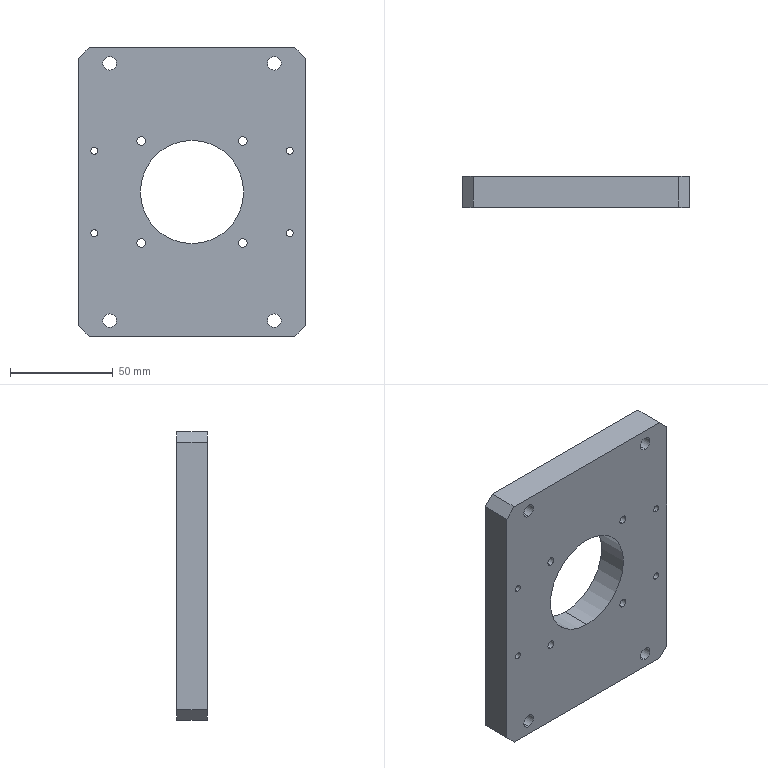Part | SolidWorks | features BaseBody 1 | 1 solid | 48 faces | box 110 x 15 x 140 mm | volume 195510 mm3 | cylinder 34 | plane 14 | commonest cylinder face diameters 3.3 x8 4.2 x8 6.6 x8 11 x8 50.2 x2
STEP:
#1=CARTESIAN_POINT('',(-47.5,0.,-21.65));
#2=VERTEX_POINT('',#1);
#3=CARTESIAN_POINT('',(-47.5,0.,-18.35));
#4=VERTEX_POINT('',#3);
#5=CARTESIAN_POINT('',(-47.5,0.,-20.));
#6=DIRECTION('',(0.,1.,0.));
#7=DIRECTION('',(0.,0.,1.));
#8=AXIS2_PLACEMENT_3D('',#5,#6,#7);
#9=CIRCLE('',#8,1.65);
#10=EDGE_CURVE('',#2,#4,#9,.T.);
#11=ORIENTED_EDGE('',*,*,#10,.F.);
#12=CARTESIAN_POINT('',(-47.5,15.,-21.65));
#13=VERTEX_POINT('',#12);
#14=CARTESIAN_POINT('',(-47.5,15.,-21.65));
#15=DIRECTION('',(0.,1.,0.));
#16=VECTOR('',#15,1000.);
#17=LINE('',#14,#16);
#18=EDGE_CURVE('',#2,#13,#17,.T.);
#19=ORIENTED_EDGE('',*,*,#18,.T.);
#20=CARTESIAN_POINT('',(-47.5,15.,-18.35));
#21=VERTEX_POINT('',#20);
#22=CARTESIAN_POINT('',(-47.5,15.,-20.));
#23=DIRECTION('',(0.,1.,0.));
#24=DIRECTION('',(0.,0.,1.));
#25=AXIS2_PLACEMENT_3D('',#22,#23,#24);
#26=CIRCLE('',#25,1.65);
#27=EDGE_CURVE('',#13,#21,#26,.T.);
#28=ORIENTED_EDGE('',*,*,#27,.T.);
#29=CARTESIAN_POINT('',(-47.5,15.,-18.35));
#30=DIRECTION('',(0.,1.,0.));
#31=VECTOR('',#30,1000.);
#32=LINE('',#29,#31);
#33=EDGE_CURVE('',#4,#21,#32,.T.);
#34=ORIENTED_EDGE('',*,*,#33,.F.);
#35=EDGE_LOOP('',(#11,#19,#28,#34));
#36=FACE_OUTER_BOUND('',#35,.T.);
#37=CARTESIAN_POINT('',(-47.5,15.,-20.));
#38=DIRECTION('',(0.,1.,0.));
#39=DIRECTION('',(0.,0.,1.));
#40=AXIS2_PLACEMENT_3D('',#37,#38,#39);
#41=CYLINDRICAL_SURFACE('',#40,1.65);
#42=ADVANCED_FACE('',(#36),#41,.F.);
#43=CARTESIAN_POINT('',(47.5,0.,-21.65));
#44=VERTEX_POINT('',#43);
#45=CARTESIAN_POINT('',(47.5,0.,-18.35));
#46=VERTEX_POINT('',#45);
#47=CARTESIAN_POINT('',(47.5,0.,-20.));
#48=DIRECTION('',(0.,1.,0.));
#49=DIRECTION('',(0.,0.,1.));
#50=AXIS2_PLACEMENT_3D('',#47,#48,#49);
#51=CIRCLE('',#50,1.65);
#52=EDGE_CURVE('',#44,#46,#51,.T.);
#53=ORIENTED_EDGE('',*,*,#52,.F.);
#54=CARTESIAN_POINT('',(47.5,15.,-21.65));
#55=VERTEX_POINT('',#54);
#56=CARTESIAN_POINT('',(47.5,15.,-21.65));
#57=DIRECTION('',(0.,1.,0.));
#58=VECTOR('',#57,1000.);
#59=LINE('',#56,#58);
#60=EDGE_CURVE('',#44,#55,#59,.T.);
#61=ORIENTED_EDGE('',*,*,#60,.T.);
#62=CARTESIAN_POINT('',(47.5,15.,-18.35));
#63=VERTEX_POINT('',#62);
#64=CARTESIAN_POINT('',(47.5,15.,-20.));
#65=DIRECTION('',(0.,1.,0.));
#66=DIRECTION('',(0.,0.,1.));
#67=AXIS2_PLACEMENT_3D('',#64,#65,#66);
#68=CIRCLE('',#67,1.65);
#69=EDGE_CURVE('',#55,#63,#68,.T.);
#70=ORIENTED_EDGE('',*,*,#69,.T.);
#71=CARTESIAN_POINT('',(47.5,15.,-18.35));
#72=DIRECTION('',(0.,1.,0.));
#73=VECTOR('',#72,1000.);
#74=LINE('',#71,#73);
#75=EDGE_CURVE('',#46,#63,#74,.T.);
#76=ORIENTED_EDGE('',*,*,#75,.F.);
#77=EDGE_LOOP('',(#53,#61,#70,#76));
#78=FACE_OUTER_BOUND('',#77,.T.);
#79=CARTESIAN_POINT('',(47.5,15.,-20.));
#80=DIRECTION('',(0.,1.,0.));
#81=DIRECTION('',(0.,0.,1.));
#82=AXIS2_PLACEMENT_3D('',#79,#80,#81);
#83=CYLINDRICAL_SURFACE('',#82,1.65);
#84=ADVANCED_FACE('',(#78),#83,.F.);
#85=CARTESIAN_POINT('',(-47.5,0.,18.35));
#86=VERTEX_POINT('',#85);
#87=CARTESIAN_POINT('',(-47.5,0.,21.65));
#88=VERTEX_POINT('',#87);
#89=CARTESIAN_POINT('',(-47.5,0.,20.));
#90=DIRECTION('',(0.,1.,0.));
#91=DIRECTION('',(0.,0.,1.));
#92=AXIS2_PLACEMENT_3D('',#89,#90,#91);
#93=CIRCLE('',#92,1.65);
#94=EDGE_CURVE('',#86,#88,#93,.T.);
#95=ORIENTED_EDGE('',*,*,#94,.F.);
#96=CARTESIAN_POINT('',(-47.5,15.,18.35));
#97=VERTEX_POINT('',#96);
#98=CARTESIAN_POINT('',(-47.5,15.,18.35));
#99=DIRECTION('',(0.,1.,0.));
#100=VECTOR('',#99,1000.);
#101=LINE('',#98,#100);
#102=EDGE_CURVE('',#86,#97,#101,.T.);
#103=ORIENTED_EDGE('',*,*,#102,.T.);
#104=CARTESIAN_POINT('',(-47.5,15.,21.65));
#105=VERTEX_POINT('',#104);
#106=CARTESIAN_POINT('',(-47.5,15.,20.));
#107=DIRECTION('',(0.,1.,0.));
#108=DIRECTION('',(0.,0.,1.));
#109=AXIS2_PLACEMENT_3D('',#106,#107,#108);
#110=CIRCLE('',#109,1.65);
#111=EDGE_CURVE('',#97,#105,#110,.T.);
#112=ORIENTED_EDGE('',*,*,#111,.T.);
#113=CARTESIAN_POINT('',(-47.5,15.,21.65));
#114=DIRECTION('',(0.,1.,0.));
#115=VECTOR('',#114,1000.);
#116=LINE('',#113,#115);
#117=EDGE_CURVE('',#88,#105,#116,.T.);
#118=ORIENTED_EDGE('',*,*,#117,.F.);
#119=EDGE_LOOP('',(#95,#103,#112,#118));
#120=FACE_OUTER_BOUND('',#119,.T.);
#121=CARTESIAN_POINT('',(-47.5,15.,20.));
#122=DIRECTION('',(0.,1.,0.));
#123=DIRECTION('',(0.,0.,1.));
#124=AXIS2_PLACEMENT_3D('',#121,#122,#123);
#125=CYLINDRICAL_SURFACE('',#124,1.65);
#126=ADVANCED_FACE('',(#120),#125,.F.);
#127=CARTESIAN_POINT('',(47.5,0.,18.35));
#128=VERTEX_POINT('',#127);
#129=CARTESIAN_POINT('',(47.5,0.,21.65));
#130=VERTEX_POINT('',#129);
#131=CARTESIAN_POINT('',(47.5,0.,20.));
#132=DIRECTION('',(0.,1.,0.));
#133=DIRECTION('',(0.,0.,1.));
#134=AXIS2_PLACEMENT_3D('',#131,#132,#133);
#135=CIRCLE('',#134,1.65);
#136=EDGE_CURVE('',#128,#130,#135,.T.);
#137=ORIENTED_EDGE('',*,*,#136,.F.);
#138=CARTESIAN_POINT('',(47.5,15.,18.35));
#139=VERTEX_POINT('',#138);
#140=CARTESIAN_POINT('',(47.5,15.,18.35));
#141=DIRECTION('',(0.,1.,0.));
#142=VECTOR('',#141,1000.);
#143=LINE('',#140,#142);
#144=EDGE_CURVE('',#128,#139,#143,.T.);
#145=ORIENTED_EDGE('',*,*,#144,.T.);
#146=CARTESIAN_POINT('',(47.5,15.,21.65));
#147=VERTEX_POINT('',#146);
#148=CARTESIAN_POINT('',(47.5,15.,20.));
#149=DIRECTION('',(0.,1.,0.));
#150=DIRECTION('',(0.,0.,1.));
#151=AXIS2_PLACEMENT_3D('',#148,#149,#150);
#152=CIRCLE('',#151,1.65);
#153=EDGE_CURVE('',#139,#147,#152,.T.);
#154=ORIENTED_EDGE('',*,*,#153,.T.);
#155=CARTESIAN_POINT('',(47.5,15.,21.65));
#156=DIRECTION('',(0.,1.,0.));
#157=VECTOR('',#156,1000.);
#158=LINE('',#155,#157);
#159=EDGE_CURVE('',#130,#147,#158,.T.);
#160=ORIENTED_EDGE('',*,*,#159,.F.);
#161=EDGE_LOOP('',(#137,#145,#154,#160));
#162=FACE_OUTER_BOUND('',#161,.T.);
#163=CARTESIAN_POINT('',(47.5,15.,20.));
#164=DIRECTION('',(0.,1.,0.));
#165=DIRECTION('',(0.,0.,1.));
#166=AXIS2_PLACEMENT_3D('',#163,#164,#165);
#167=CYLINDRICAL_SURFACE('',#166,1.65);
#168=ADVANCED_FACE('',(#162),#167,.F.);
#169=CARTESIAN_POINT('',(-40.,8.2,-68.));
#170=VERTEX_POINT('',#169);
#171=CARTESIAN_POINT('',(-40.,8.2,-57.));
#172=VERTEX_POINT('',#171);
#173=CARTESIAN_POINT('',(-40.,8.2,-62.5));
#174=DIRECTION('',(0.,1.,0.));
#175=DIRECTION('',(0.,0.,1.));
#176=AXIS2_PLACEMENT_3D('',#173,#174,#175);
#177=CIRCLE('',#176,5.5);
#178=EDGE_CURVE('',#170,#172,#177,.T.);
#179=ORIENTED_EDGE('',*,*,#178,.F.);
#180=CARTESIAN_POINT('',(-40.,15.,-68.));
#181=VERTEX_POINT('',#180);
#182=CARTESIAN_POINT('',(-40.,15.,-68.));
#183=DIRECTION('',(0.,1.,0.));
#184=VECTOR('',#183,1000.);
#185=LINE('',#182,#184);
#186=EDGE_CURVE('',#170,#181,#185,.T.);
#187=ORIENTED_EDGE('',*,*,#186,.T.);
#188=CARTESIAN_POINT('',(-40.,15.,-57.));
#189=VERTEX_POINT('',#188);
#190=CARTESIAN_POINT('',(-40.,15.,-62.5));
#191=DIRECTION('',(0.,1.,0.));
#192=DIRECTION('',(0.,0.,1.));
#193=AXIS2_PLACEMENT_3D('',#190,#191,#192);
#194=CIRCLE('',#193,5.5);
#195=EDGE_CURVE('',#181,#189,#194,.T.);
#196=ORIENTED_EDGE('',*,*,#195,.T.);
#197=CARTESIAN_POINT('',(-40.,15.,-57.));
#198=DIRECTION('',(0.,1.,0.));
#199=VECTOR('',#198,1000.);
#200=LINE('',#197,#199);
#201=EDGE_CURVE('',#172,#189,#200,.T.);
#202=ORIENTED_EDGE('',*,*,#201,.F.);
#203=EDGE_LOOP('',(#179,#187,#196,#202));
#204=FACE_OUTER_BOUND('',#203,.T.);
#205=CARTESIAN_POINT('',(-40.,15.,-62.5));
#206=DIRECTION('',(0.,1.,0.));
#207=DIRECTION('',(0.,0.,1.));
#208=AXIS2_PLACEMENT_3D('',#205,#206,#207);
#209=CYLINDRICAL_SURFACE('',#208,5.5);
#210=ADVANCED_FACE('',(#204),#209,.F.);
#211=CARTESIAN_POINT('',(-40.,0.,-65.8));
#212=VERTEX_POINT('',#211);
#213=CARTESIAN_POINT('',(-40.,0.,-59.2));
#214=VERTEX_POINT('',#213);
#215=CARTESIAN_POINT('',(-40.,0.,-62.5));
#216=DIRECTION('',(0.,1.,0.));
#217=DIRECTION('',(0.,0.,1.));
#218=AXIS2_PLACEMENT_3D('',#215,#216,#217);
#219=CIRCLE('',#218,3.3);
#220=EDGE_CURVE('',#212,#214,#219,.T.);
#221=ORIENTED_EDGE('',*,*,#220,.F.);
#222=CARTESIAN_POINT('',(-40.,8.2,-65.8));
#223=VERTEX_POINT('',#222);
#224=CARTESIAN_POINT('',(-40.,15.,-65.8));
#225=DIRECTION('',(0.,1.,0.));
#226=VECTOR('',#225,1000.);
#227=LINE('',#224,#226);
#228=EDGE_CURVE('',#212,#223,#227,.T.);
#229=ORIENTED_EDGE('',*,*,#228,.T.);
#230=CARTESIAN_POINT('',(-40.,8.2,-59.2));
#231=VERTEX_POINT('',#230);
#232=CARTESIAN_POINT('',(-40.,8.2,-62.5));
#233=DIRECTION('',(0.,1.,0.));
#234=DIRECTION('',(0.,0.,1.));
#235=AXIS2_PLACEMENT_3D('',#232,#233,#234);
#236=CIRCLE('',#235,3.3);
#237=EDGE_CURVE('',#223,#231,#236,.T.);
#238=ORIENTED_EDGE('',*,*,#237,.T.);
#239=CARTESIAN_POINT('',(-40.,15.,-59.2));
#240=DIRECTION('',(0.,1.,0.));
#241=VECTOR('',#240,1000.);
#242=LINE('',#239,#241);
#243=EDGE_CURVE('',#214,#231,#242,.T.);
#244=ORIENTED_EDGE('',*,*,#243,.F.);
#245=EDGE_LOOP('',(#221,#229,#238,#244));
#246=FACE_OUTER_BOUND('',#245,.T.);
#247=CARTESIAN_POINT('',(-40.,15.,-62.5));
#248=DIRECTION('',(0.,1.,0.));
#249=DIRECTION('',(0.,0.,1.));
#250=AXIS2_PLACEMENT_3D('',#247,#248,#249);
#251=CYLINDRICAL_SURFACE('',#250,3.3);
#252=ADVANCED_FACE('',(#246),#251,.F.);
#253=CARTESIAN_POINT('',(-40.,8.2,57.));
#254=VERTEX_POINT('',#253);
#255=CARTESIAN_POINT('',(-40.,8.2,68.));
#256=VERTEX_POINT('',#255);
#257=CARTESIAN_POINT('',(-40.,8.2,62.5));
#258=DIRECTION('',(0.,1.,0.));
#259=DIRECTION('',(0.,0.,1.));
#260=AXIS2_PLACEMENT_3D('',#257,#258,#259);
#261=CIRCLE('',#260,5.5);
#262=EDGE_CURVE('',#254,#256,#261,.T.);
#263=ORIENTED_EDGE('',*,*,#262,.F.);
#264=CARTESIAN_POINT('',(-40.,15.,57.));
#265=VERTEX_POINT('',#264);
#266=CARTESIAN_POINT('',(-40.,15.,57.));
#267=DIRECTION('',(0.,1.,0.));
#268=VECTOR('',#267,1000.);
#269=LINE('',#266,#268);
#270=EDGE_CURVE('',#254,#265,#269,.T.);
#271=ORIENTED_EDGE('',*,*,#270,.T.);
#272=CARTESIAN_POINT('',(-40.,15.,68.));
#273=VERTEX_POINT('',#272);
#274=CARTESIAN_POINT('',(-40.,15.,62.5));
#275=DIRECTION('',(0.,1.,0.));
#276=DIRECTION('',(0.,0.,1.));
#277=AXIS2_PLACEMENT_3D('',#274,#275,#276);
#278=CIRCLE('',#277,5.5);
#279=EDGE_CURVE('',#265,#273,#278,.T.);
#280=ORIENTED_EDGE('',*,*,#279,.T.);
#281=CARTESIAN_POINT('',(-40.,15.,68.));
#282=DIRECTION('',(0.,1.,0.));
#283=VECTOR('',#282,1000.);
#284=LINE('',#281,#283);
#285=EDGE_CURVE('',#256,#273,#284,.T.);
#286=ORIENTED_EDGE('',*,*,#285,.F.);
#287=EDGE_LOOP('',(#263,#271,#280,#286));
#288=FACE_OUTER_BOUND('',#287,.T.);
#289=CARTESIAN_POINT('',(-40.,15.,62.5));
#290=DIRECTION('',(0.,1.,0.));
#291=DIRECTION('',(0.,0.,1.));
#292=AXIS2_PLACEMENT_3D('',#289,#290,#291);
#293=CYLINDRICAL_SURFACE('',#292,5.5);
#294=ADVANCED_FACE('',(#288),#293,.F.);
#295=CARTESIAN_POINT('',(-40.,0.,59.2));
#296=VERTEX_POINT('',#295);
#297=CARTESIAN_POINT('',(-40.,0.,65.8));
#298=VERTEX_POINT('',#297);
#299=CARTESIAN_POINT('',(-40.,0.,62.5));
#300=DIRECTION('',(0.,1.,0.));
#301=DIRECTION('',(0.,0.,1.));
#302=AXIS2_PLACEMENT_3D('',#299,#300,#301);
#303=CIRCLE('',#302,3.3);
#304=EDGE_CURVE('',#296,#298,#303,.T.);
#305=ORIENTED_EDGE('',*,*,#304,.F.);
#306=CARTESIAN_POINT('',(-40.,8.2,59.2));
#307=VERTEX_POINT('',#306);
#308=CARTESIAN_POINT('',(-40.,15.,59.2));
#309=DIRECTION('',(0.,1.,0.));
#310=VECTOR('',#309,1000.);
#311=LINE('',#308,#310);
#312=EDGE_CURVE('',#296,#307,#311,.T.);
#313=ORIENTED_EDGE('',*,*,#312,.T.);
#314=CARTESIAN_POINT('',(-40.,8.2,65.8));
#315=VERTEX_POINT('',#314);
#316=CARTESIAN_POINT('',(-40.,8.2,62.5));
#317=DIRECTION('',(0.,1.,0.));
#318=DIRECTION('',(0.,0.,1.));
#319=AXIS2_PLACEMENT_3D('',#316,#317,#318);
#320=CIRCLE('',#319,3.3);
#321=EDGE_CURVE('',#307,#315,#320,.T.);
#322=ORIENTED_EDGE('',*,*,#321,.T.);
#323=CARTESIAN_POINT('',(-40.,15.,65.8));
#324=DIRECTION('',(0.,1.,0.));
#325=VECTOR('',#324,1000.);
#326=LINE('',#323,#325);
#327=EDGE_CURVE('',#298,#315,#326,.T.);
#328=ORIENTED_EDGE('',*,*,#327,.F.);
#329=EDGE_LOOP('',(#305,#313,#322,#328));
#330=FACE_OUTER_BOUND('',#329,.T.);
#331=CARTESIAN_POINT('',(-40.,15.,62.5));
#332=DIRECTION('',(0.,1.,0.));
#333=DIRECTION('',(0.,0.,1.));
#334=AXIS2_PLACEMENT_3D('',#331,#332,#333);
#335=CYLINDRICAL_SURFACE('',#334,3.3);
#336=ADVANCED_FACE('',(#330),#335,.F.);
#337=CARTESIAN_POINT('',(40.,8.2,57.));
#338=VERTEX_POINT('',#337);
#339=CARTESIAN_POINT('',(40.,8.2,68.));
#340=VERTEX_POINT('',#339);
#341=CARTESIAN_POINT('',(40.,8.2,62.5));
#342=DIRECTION('',(0.,1.,0.));
#343=DIRECTION('',(0.,0.,1.));
#344=AXIS2_PLACEMENT_3D('',#341,#342,#343);
#345=CIRCLE('',#344,5.5);
#346=EDGE_CURVE('',#338,#340,#345,.T.);
#347=ORIENTED_EDGE('',*,*,#346,.F.);
#348=CARTESIAN_POINT('',(40.,15.,57.));
#349=VERTEX_POINT('',#348);
#350=CARTESIAN_POINT('',(40.,15.,57.));
#351=DIRECTION('',(0.,1.,0.));
#352=VECTOR('',#351,1000.);
#353=LINE('',#350,#352);
#354=EDGE_CURVE('',#338,#349,#353,.T.);
#355=ORIENTED_EDGE('',*,*,#354,.T.);
#356=CARTESIAN_POINT('',(40.,15.,68.));
#357=VERTEX_POINT('',#356);
#358=CARTESIAN_POINT('',(40.,15.,62.5));
#359=DIRECTION('',(0.,1.,0.));
#360=DIRECTION('',(0.,0.,1.));
#361=AXIS2_PLACEMENT_3D('',#358,#359,#360);
#362=CIRCLE('',#361,5.5);
#363=EDGE_CURVE('',#349,#357,#362,.T.);
#364=ORIENTED_EDGE('',*,*,#363,.T.);
#365=CARTESIAN_POINT('',(40.,15.,68.));
#366=DIRECTION('',(0.,1.,0.));
#367=VECTOR('',#366,1000.);
#368=LINE('',#365,#367);
#369=EDGE_CURVE('',#340,#357,#368,.T.);
#370=ORIENTED_EDGE('',*,*,#369,.F.);
#371=EDGE_LOOP('',(#347,#355,#364,#370));
#372=FACE_OUTER_BOUND('',#371,.T.);
#373=CARTESIAN_POINT('',(40.,15.,62.5));
#374=DIRECTION('',(0.,1.,0.));
#375=DIRECTION('',(0.,0.,1.));
#376=AXIS2_PLACEMENT_3D('',#373,#374,#375);
#377=CYLINDRICAL_SURFACE('',#376,5.5);
#378=ADVANCED_FACE('',(#372),#377,.F.);
#379=CARTESIAN_POINT('',(40.,0.,59.2));
#380=VERTEX_POINT('',#379);
#381=CARTESIAN_POINT('',(40.,0.,65.8));
#382=VERTEX_POINT('',#381);
#383=CARTESIAN_POINT('',(40.,0.,62.5));
#384=DIRECTION('',(0.,1.,0.));
#385=DIRECTION('',(0.,0.,1.));
#386=AXIS2_PLACEMENT_3D('',#383,#384,#385);
#387=CIRCLE('',#386,3.3);
#388=EDGE_CURVE('',#380,#382,#387,.T.);
#389=ORIENTED_EDGE('',*,*,#388,.F.);
#390=CARTESIAN_POINT('',(40.,8.2,59.2));
#391=VERTEX_POINT('',#390);
#392=CARTESIAN_POINT('',(40.,15.,59.2));
#393=DIRECTION('',(0.,1.,0.));
#394=VECTOR('',#393,1000.);
#395=LINE('',#392,#394);
#396=EDGE_CURVE('',#380,#391,#395,.T.);
#397=ORIENTED_EDGE('',*,*,#396,.T.);
#398=CARTESIAN_POINT('',(40.,8.2,65.8));
#399=VERTEX_POINT('',#398);
#400=CARTESIAN_POINT('',(40.,8.2,62.5));
#401=DIRECTION('',(0.,1.,0.));
#402=DIRECTION('',(0.,0.,1.));
#403=AXIS2_PLACEMENT_3D('',#400,#401,#402);
#404=CIRCLE('',#403,3.3);
#405=EDGE_CURVE('',#391,#399,#404,.T.);
#406=ORIENTED_EDGE('',*,*,#405,.T.);
#407=CARTESIAN_POINT('',(40.,15.,65.8));
#408=DIRECTION('',(0.,1.,0.));
#409=VECTOR('',#408,1000.);
#410=LINE('',#407,#409);
#411=EDGE_CURVE('',#382,#399,#410,.T.);
#412=ORIENTED_EDGE('',*,*,#411,.F.);
#413=EDGE_LOOP('',(#389,#397,#406,#412));
#414=FACE_OUTER_BOUND('',#413,.T.);
#415=CARTESIAN_POINT('',(40.,15.,62.5));
#416=DIRECTION('',(0.,1.,0.));
#417=DIRECTION('',(0.,0.,1.));
#418=AXIS2_PLACEMENT_3D('',#415,#416,#417);
#419=CYLINDRICAL_SURFACE('',#418,3.3);
#420=ADVANCED_FACE('',(#414),#419,.F.);
#421=CARTESIAN_POINT('',(40.,8.2,-68.));
#422=VERTEX_POINT('',#421);
#423=CARTESIAN_POINT('',(40.,8.2,-57.));
#424=VERTEX_POINT('',#423);
#425=CARTESIAN_POINT('',(40.,8.2,-62.5));
#426=DIRECTION('',(0.,1.,0.));
#427=DIRECTION('',(0.,0.,1.));
#428=AXIS2_PLACEMENT_3D('',#425,#426,#427);
#429=CIRCLE('',#428,5.5);
#430=EDGE_CURVE('',#422,#424,#429,.T.);
#431=ORIENTED_EDGE('',*,*,#430,.F.);
#432=CARTESIAN_POINT('',(40.,15.,-68.));
#433=VERTEX_POINT('',#432);
#434=CARTESIAN_POINT('',(40.,15.,-68.));
#435=DIRECTION('',(0.,1.,0.));
#436=VECTOR('',#435,1000.);
#437=LINE('',#434,#436);
#438=EDGE_CURVE('',#422,#433,#437,.T.);
#439=ORIENTED_EDGE('',*,*,#438,.T.);
#440=CARTESIAN_POINT('',(40.,15.,-57.));
#441=VERTEX_POINT('',#440);
#442=CARTESIAN_POINT('',(40.,15.,-62.5));
#443=DIRECTION('',(0.,1.,0.));
#444=DIRECTION('',(0.,0.,1.));
#445=AXIS2_PLACEMENT_3D('',#442,#443,#444);
#446=CIRCLE('',#445,5.5);
#447=EDGE_CURVE('',#433,#441,#446,.T.);
#448=ORIENTED_EDGE('',*,*,#447,.T.);
#449=CARTESIAN_POINT('',(40.,15.,-57.));
#450=DIRECTION('',(0.,1.,0.));
#451=VECTOR('',#450,1000.);
#452=LINE('',#449,#451);
#453=EDGE_CURVE('',#424,#441,#452,.T.);
#454=ORIENTED_EDGE('',*,*,#453,.F.);
#455=EDGE_LOOP('',(#431,#439,#448,#454));
#456=FACE_OUTER_BOUND('',#455,.T.);
#457=CARTESIAN_POINT('',(40.,15.,-62.5));
#458=DIRECTION('',(0.,1.,0.));
#459=DIRECTION('',(0.,0.,1.));
#460=AXIS2_PLACEMENT_3D('',#457,#458,#459);
#461=CYLINDRICAL_SURFACE('',#460,5.5);
#462=ADVANCED_FACE('',(#456),#461,.F.);
#463=CARTESIAN_POINT('',(40.,0.,-65.8));
#464=VERTEX_POINT('',#463);
#465=CARTESIAN_POINT('',(40.,0.,-59.2));
#466=VERTEX_POINT('',#465);
#467=CARTESIAN_POINT('',(40.,0.,-62.5));
#468=DIRECTION('',(0.,1.,0.));
#469=DIRECTION('',(0.,0.,1.));
#470=AXIS2_PLACEMENT_3D('',#467,#468,#469);
#471=CIRCLE('',#470,3.3);
#472=EDGE_CURVE('',#464,#466,#471,.T.);
#473=ORIENTED_EDGE('',*,*,#472,.F.);
#474=CARTESIAN_POINT('',(40.,8.2,-65.8));
#475=VERTEX_POINT('',#474);
#476=CARTESIAN_POINT('',(40.,15.,-65.8));
#477=DIRECTION('',(0.,1.,0.));
#478=VECTOR('',#477,1000.);
#479=LINE('',#476,#478);
#480=EDGE_CURVE('',#464,#475,#479,.T.);
#481=ORIENTED_EDGE('',*,*,#480,.T.);
#482=CARTESIAN_POINT('',(40.,8.2,-59.2));
#483=VERTEX_POINT('',#482);
#484=CARTESIAN_POINT('',(40.,8.2,-62.5));
#485=DIRECTION('',(0.,1.,0.));
#486=DIRECTION('',(0.,0.,1.));
#487=AXIS2_PLACEMENT_3D('',#484,#485,#486);
#488=CIRCLE('',#487,3.3);
#489=EDGE_CURVE('',#475,#483,#488,.T.);
#490=ORIENTED_EDGE('',*,*,#489,.T.);
#491=CARTESIAN_POINT('',(40.,15.,-59.2));
#492=DIRECTION('',(0.,1.,0.));
#493=VECTOR('',#492,1000.);
#494=LINE('',#491,#493);
#495=EDGE_CURVE('',#466,#483,#494,.T.);
#496=ORIENTED_EDGE('',*,*,#495,.F.);
#497=EDGE_LOOP('',(#473,#481,#490,#496));
#498=FACE_OUTER_BOUND('',#497,.T.);
#499=CARTESIAN_POINT('',(40.,15.,-62.5));
#500=DIRECTION('',(0.,1.,0.));
#501=DIRECTION('',(0.,0.,1.));
#502=AXIS2_PLACEMENT_3D('',#499,#500,#501);
#503=CYLINDRICAL_SURFACE('',#502,3.3);
#504=ADVANCED_FACE('',(#498),#503,.F.);
#505=CARTESIAN_POINT('',(-24.749,0.,-26.849));
#506=VERTEX_POINT('',#505);
#507=CARTESIAN_POINT('',(-24.749,0.,-22.649));
#508=VERTEX_POINT('',#507);
#509=CARTESIAN_POINT('',(-24.749,0.,-24.749));
#510=DIRECTION('',(0.,1.,0.));
#511=DIRECTION('',(0.,0.,1.));
#512=AXIS2_PLACEMENT_3D('',#509,#510,#511);
#513=CIRCLE('',#512,2.1);
#514=EDGE_CURVE('',#506,#508,#513,.T.);
#515=ORIENTED_EDGE('',*,*,#514,.F.);
#516=CARTESIAN_POINT('',(-24.749,15.,-26.849));
#517=VERTEX_POINT('',#516);
#518=CARTESIAN_POINT('',(-24.749,15.,-26.849));
#519=DIRECTION('',(0.,1.,0.));
#520=VECTOR('',#519,1000.);
#521=LINE('',#518,#520);
#522=EDGE_CURVE('',#506,#517,#521,.T.);
#523=ORIENTED_EDGE('',*,*,#522,.T.);
#524=CARTESIAN_POINT('',(-24.749,15.,-22.649));
#525=VERTEX_POINT('',#524);
#526=CARTESIAN_POINT('',(-24.749,15.,-24.749));
#527=DIRECTION('',(0.,1.,0.));
#528=DIRECTION('',(0.,0.,1.));
#529=AXIS2_PLACEMENT_3D('',#526,#527,#528);
#530=CIRCLE('',#529,2.1);
#531=EDGE_CURVE('',#517,#525,#530,.T.);
#532=ORIENTED_EDGE('',*,*,#531,.T.);
#533=CARTESIAN_POINT('',(-24.749,15.,-22.649));
#534=DIRECTION('',(0.,1.,0.));
#535=VECTOR('',#534,1000.);
#536=LINE('',#533,#535);
#537=EDGE_CURVE('',#508,#525,#536,.T.);
#538=ORIENTED_EDGE('',*,*,#537,.F.);
#539=EDGE_LOOP('',(#515,#523,#532,#538));
#540=FACE_OUTER_BOUND('',#539,.T.);
#541=CARTESIAN_POINT('',(-24.749,15.,-24.749));
#542=DIRECTION('',(0.,1.,0.));
#543=DIRECTION('',(0.,0.,1.));
#544=AXIS2_PLACEMENT_3D('',#541,#542,#543);
#545=CYLINDRICAL_SURFACE('',#544,2.1);
#546=ADVANCED_FACE('',(#540),#545,.F.);
#547=CARTESIAN_POINT('',(24.749,0.,22.649));
#548=VERTEX_POINT('',#547);
#549=CARTESIAN_POINT('',(24.749,0.,26.849));
#550=VERTEX_POINT('',#549);
#551=CARTESIAN_POINT('',(24.749,0.,24.749));
#552=DIRECTION('',(0.,1.,0.));
#553=DIRECTION('',(0.,0.,1.));
#554=AXIS2_PLACEMENT_3D('',#551,#552,#553);
#555=CIRCLE('',#554,2.1);
#556=EDGE_CURVE('',#548,#550,#555,.T.);
#557=ORIENTED_EDGE('',*,*,#556,.F.);
#558=CARTESIAN_POINT('',(24.749,15.,22.649));
#559=VERTEX_POINT('',#558);
#560=CARTESIAN_POINT('',(24.749,15.,22.649));
#561=DIRECTION('',(0.,1.,0.));
#562=VECTOR('',#561,1000.);
#563=LINE('',#560,#562);
#564=EDGE_CURVE('',#548,#559,#563,.T.);
#565=ORIENTED_EDGE('',*,*,#564,.T.);
#566=CARTESIAN_POINT('',(24.749,15.,26.849));
#567=VERTEX_POINT('',#566);
#568=CARTESIAN_POINT('',(24.749,15.,24.749));
#569=DIRECTION('',(0.,1.,0.));
#570=DIRECTION('',(0.,0.,1.));
#571=AXIS2_PLACEMENT_3D('',#568,#569,#570);
#572=CIRCLE('',#571,2.1);
#573=EDGE_CURVE('',#559,#567,#572,.T.);
#574=ORIENTED_EDGE('',*,*,#573,.T.);
#575=CARTESIAN_POINT('',(24.749,15.,26.849));
#576=DIRECTION('',(0.,1.,0.));
#577=VECTOR('',#576,1000.);
#578=LINE('',#575,#577);
#579=EDGE_CURVE('',#550,#567,#578,.T.);
#580=ORIENTED_EDGE('',*,*,#579,.F.);
#581=EDGE_LOOP('',(#557,#565,#574,#580));
#582=FACE_OUTER_BOUND('',#581,.T.);
#583=CARTESIAN_POINT('',(24.749,15.,24.749));
#584=DIRECTION('',(0.,1.,0.));
#585=DIRECTION('',(0.,0.,1.));
#586=AXIS2_PLACEMENT_3D('',#583,#584,#585);
#587=CYLINDRICAL_SURFACE('',#586,2.1);
#588=ADVANCED_FACE('',(#582),#587,.F.);
#589=CARTESIAN_POINT('',(24.749,0.,-26.849));
#590=VERTEX_POINT('',#589);
#591=CARTESIAN_POINT('',(24.749,0.,-22.649));
#592=VERTEX_POINT('',#591);
#593=CARTESIAN_POINT('',(24.749,0.,-24.749));
#594=DIRECTION('',(0.,1.,0.));
#595=DIRECTION('',(0.,0.,1.));
#596=AXIS2_PLACEMENT_3D('',#593,#594,#595);
#597=CIRCLE('',#596,2.1);
#598=EDGE_CURVE('',#590,#592,#597,.T.);
#599=ORIENTED_EDGE('',*,*,#598,.F.);
#600=CARTESIAN_POINT('',(24.749,15.,-26.849));
#601=VERTEX_POINT('',#600);
#602=CARTESIAN_POINT('',(24.749,15.,-26.849));
#603=DIRECTION('',(0.,1.,0.));
#604=VECTOR('',#603,1000.);
#605=LINE('',#602,#604);
#606=EDGE_CURVE('',#590,#601,#605,.T.);
#607=ORIENTED_EDGE('',*,*,#606,.T.);
#608=CARTESIAN_POINT('',(24.749,15.,-22.649));
#609=VERTEX_POINT('',#608);
#610=CARTESIAN_POINT('',(24.749,15.,-24.749));
#611=DIRECTION('',(0.,1.,0.));
#612=DIRECTION('',(0.,0.,1.));
#613=AXIS2_PLACEMENT_3D('',#610,#611,#612);
#614=CIRCLE('',#613,2.1);
#615=EDGE_CURVE('',#601,#609,#614,.T.);
#616=ORIENTED_EDGE('',*,*,#615,.T.);
#617=CARTESIAN_POINT('',(24.749,15.,-22.649));
#618=DIRECTION('',(0.,1.,0.));
#619=VECTOR('',#618,1000.);
#620=LINE('',#617,#619);
#621=EDGE_CURVE('',#592,#609,#620,.T.);
#622=ORIENTED_EDGE('',*,*,#621,.F.);
#623=EDGE_LOOP('',(#599,#607,#616,#622));
#624=FACE_OUTER_BOUND('',#623,.T.);
#625=CARTESIAN_POINT('',(24.749,15.,-24.749));
#626=DIRECTION('',(0.,1.,0.));
#627=DIRECTION('',(0.,0.,1.));
#628=AXIS2_PLACEMENT_3D('',#625,#626,#627);
#629=CYLINDRICAL_SURFACE('',#628,2.1);
#630=ADVANCED_FACE('',(#624),#629,.F.);
#631=CARTESIAN_POINT('',(-24.749,0.,22.649));
#632=VERTEX_POINT('',#631);
#633=CARTESIAN_POINT('',(-24.749,0.,26.849));
#634=VERTEX_POINT('',#633);
#635=CARTESIAN_POINT('',(-24.749,0.,24.749));
#636=DIRECTION('',(0.,1.,0.));
#637=DIRECTION('',(0.,0.,1.));
#638=AXIS2_PLACEMENT_3D('',#635,#636,#637);
#639=CIRCLE('',#638,2.1);
#640=EDGE_CURVE('',#632,#634,#639,.T.);
#641=ORIENTED_EDGE('',*,*,#640,.F.);
#642=CARTESIAN_POINT('',(-24.749,15.,22.649));
#643=VERTEX_POINT('',#642);
#644=CARTESIAN_POINT('',(-24.749,15.,22.649));
#645=DIRECTION('',(0.,1.,0.));
#646=VECTOR('',#645,1000.);
#647=LINE('',#644,#646);
#648=EDGE_CURVE('',#632,#643,#647,.T.);
#649=ORIENTED_EDGE('',*,*,#648,.T.);
#650=CARTESIAN_POINT('',(-24.749,15.,26.849));
#651=VERTEX_POINT('',#650);
#652=CARTESIAN_POINT('',(-24.749,15.,24.749));
#653=DIRECTION('',(0.,1.,0.));
#654=DIRECTION('',(0.,0.,1.));
#655=AXIS2_PLACEMENT_3D('',#652,#653,#654);
#656=CIRCLE('',#655,2.1);
#657=EDGE_CURVE('',#643,#651,#656,.T.);
#658=ORIENTED_EDGE('',*,*,#657,.T.);
#659=CARTESIAN_POINT('',(-24.749,15.,26.849));
#660=DIRECTION('',(0.,1.,0.));
#661=VECTOR('',#660,1000.);
#662=LINE('',#659,#661);
#663=EDGE_CURVE('',#634,#651,#662,.T.);
#664=ORIENTED_EDGE('',*,*,#663,.F.);
#665=EDGE_LOOP('',(#641,#649,#658,#664));
#666=FACE_OUTER_BOUND('',#665,.T.);
#667=CARTESIAN_POINT('',(-24.749,15.,24.749));
#668=DIRECTION('',(0.,1.,0.));
#669=DIRECTION('',(0.,0.,1.));
#670=AXIS2_PLACEMENT_3D('',#667,#668,#669);
#671=CYLINDRICAL_SURFACE('',#670,2.1);
#672=ADVANCED_FACE('',(#666),#671,.F.);
#673=CARTESIAN_POINT('',(0.,0.,-25.1));
#674=VERTEX_POINT('',#673);
#675=CARTESIAN_POINT('',(0.,0.,25.1));
#676=VERTEX_POINT('',#675);
#677=CARTESIAN_POINT('',(0.,0.,0.));
#678=DIRECTION('',(0.,1.,0.));
#679=DIRECTION('',(0.,0.,1.));
#680=AXIS2_PLACEMENT_3D('',#677,#678,#679);
#681=CIRCLE('',#680,25.1);
#682=EDGE_CURVE('',#674,#676,#681,.T.);
#683=ORIENTED_EDGE('',*,*,#682,.F.);
#684=CARTESIAN_POINT('',(0.,15.,-25.1));
#685=VERTEX_POINT('',#684);
#686=CARTESIAN_POINT('',(0.,0.,-25.1));
#687=DIRECTION('',(0.,1.,0.));
#688=VECTOR('',#687,1000.);
#689=LINE('',#686,#688);
#690=EDGE_CURVE('',#674,#685,#689,.T.);
#691=ORIENTED_EDGE('',*,*,#690,.T.);
#692=CARTESIAN_POINT('',(0.,15.,25.1));
#693=VERTEX_POINT('',#692);
#694=CARTESIAN_POINT('',(0.,15.,0.));
#695=DIRECTION('',(0.,1.,0.));
#696=DIRECTION('',(0.,0.,1.));
#697=AXIS2_PLACEMENT_3D('',#694,#695,#696);
#698=CIRCLE('',#697,25.1);
#699=EDGE_CURVE('',#685,#693,#698,.T.);
#700=ORIENTED_EDGE('',*,*,#699,.T.);
#701=CARTESIAN_POINT('',(0.,0.,25.1));
#702=DIRECTION('',(0.,1.,0.));
#703=VECTOR('',#702,1000.);
#704=LINE('',#701,#703);
#705=EDGE_CURVE('',#676,#693,#704,.T.);
#706=ORIENTED_EDGE('',*,*,#705,.F.);
#707=EDGE_LOOP('',(#683,#691,#700,#706));
#708=FACE_OUTER_BOUND('',#707,.T.);
#709=CARTESIAN_POINT('',(0.,0.,0.));
#710=DIRECTION('',(0.,1.,0.));
#711=DIRECTION('',(0.,0.,1.));
#712=AXIS2_PLACEMENT_3D('',#709,#710,#711);
#713=CYLINDRICAL_SURFACE('',#712,25.1);
#714=ADVANCED_FACE('',(#708),#713,.F.);
#715=CARTESIAN_POINT('',(-40.,8.2,-62.5));
#716=DIRECTION('',(0.,1.,0.));
#717=DIRECTION('',(0.,0.,1.));
#718=AXIS2_PLACEMENT_3D('',#715,#716,#717);
#719=CIRCLE('',#718,3.3);
#720=EDGE_CURVE('',#231,#223,#719,.T.);
#721=ORIENTED_EDGE('',*,*,#720,.F.);
#722=ORIENTED_EDGE('',*,*,#237,.F.);
#723=EDGE_LOOP('',(#721,#722));
#724=FACE_BOUND('',#723,.T.);
#725=CARTESIAN_POINT('',(-40.,8.2,-62.5));
#726=DIRECTION('',(0.,1.,0.));
#727=DIRECTION('',(0.,0.,1.));
#728=AXIS2_PLACEMENT_3D('',#725,#726,#727);
#729=CIRCLE('',#728,5.5);
#730=EDGE_CURVE('',#172,#170,#729,.T.);
#731=ORIENTED_EDGE('',*,*,#730,.T.);
#732=ORIENTED_EDGE('',*,*,#178,.T.);
#733=EDGE_LOOP('',(#731,#732));
#734=FACE_OUTER_BOUND('',#733,.T.);
#735=CARTESIAN_POINT('',(-36.7,8.2,-62.5));
#736=DIRECTION('',(0.,-1.,0.));
#737=DIRECTION('',(0.,0.,-1.));
#738=AXIS2_PLACEMENT_3D('',#735,#736,#737);
#739=PLANE('',#738);
#740=ADVANCED_FACE('',(#724,#734),#739,.F.);
#741=CARTESIAN_POINT('',(-40.,8.2,62.5));
#742=DIRECTION('',(0.,1.,0.));
#743=DIRECTION('',(0.,0.,1.));
#744=AXIS2_PLACEMENT_3D('',#741,#742,#743);
#745=CIRCLE('',#744,3.3);
#746=EDGE_CURVE('',#315,#307,#745,.T.);
#747=ORIENTED_EDGE('',*,*,#746,.F.);
#748=ORIENTED_EDGE('',*,*,#321,.F.);
#749=EDGE_LOOP('',(#747,#748));
#750=FACE_BOUND('',#749,.T.);
#751=CARTESIAN_POINT('',(-40.,8.2,62.5));
#752=DIRECTION('',(0.,1.,0.));
#753=DIRECTION('',(0.,0.,1.));
#754=AXIS2_PLACEMENT_3D('',#751,#752,#753);
#755=CIRCLE('',#754,5.5);
#756=EDGE_CURVE('',#256,#254,#755,.T.);
#757=ORIENTED_EDGE('',*,*,#756,.T.);
#758=ORIENTED_EDGE('',*,*,#262,.T.);
#759=EDGE_LOOP('',(#757,#758));
#760=FACE_OUTER_BOUND('',#759,.T.);
#761=CARTESIAN_POINT('',(-36.7,8.2,62.5));
#762=DIRECTION('',(0.,-1.,0.));
#763=DIRECTION('',(0.,0.,-1.));
#764=AXIS2_PLACEMENT_3D('',#761,#762,#763);
#765=PLANE('',#764);
#766=ADVANCED_FACE('',(#750,#760),#765,.F.);
#767=CARTESIAN_POINT('',(40.,8.2,62.5));
#768=DIRECTION('',(0.,1.,0.));
#769=DIRECTION('',(0.,0.,1.));
#770=AXIS2_PLACEMENT_3D('',#767,#768,#769);
#771=CIRCLE('',#770,3.3);
#772=EDGE_CURVE('',#399,#391,#771,.T.);
#773=ORIENTED_EDGE('',*,*,#772,.F.);
#774=ORIENTED_EDGE('',*,*,#405,.F.);
#775=EDGE_LOOP('',(#773,#774));
#776=FACE_BOUND('',#775,.T.);
#777=CARTESIAN_POINT('',(40.,8.2,62.5));
#778=DIRECTION('',(0.,1.,0.));
#779=DIRECTION('',(0.,0.,1.));
#780=AXIS2_PLACEMENT_3D('',#777,#778,#779);
#781=CIRCLE('',#780,5.5);
#782=EDGE_CURVE('',#340,#338,#781,.T.);
#783=ORIENTED_EDGE('',*,*,#782,.T.);
#784=ORIENTED_EDGE('',*,*,#346,.T.);
#785=EDGE_LOOP('',(#783,#784));
#786=FACE_OUTER_BOUND('',#785,.T.);
#787=CARTESIAN_POINT('',(43.3,8.2,62.5));
#788=DIRECTION('',(0.,-1.,0.));
#789=DIRECTION('',(0.,0.,-1.));
#790=AXIS2_PLACEMENT_3D('',#787,#788,#789);
#791=PLANE('',#790);
#792=ADVANCED_FACE('',(#776,#786),#791,.F.);
#793=CARTESIAN_POINT('',(40.,8.2,-62.5));
#794=DIRECTION('',(0.,1.,0.));
#795=DIRECTION('',(0.,0.,1.));
#796=AXIS2_PLACEMENT_3D('',#793,#794,#795);
#797=CIRCLE('',#796,3.3);
#798=EDGE_CURVE('',#483,#475,#797,.T.);
#799=ORIENTED_EDGE('',*,*,#798,.F.);
#800=ORIENTED_EDGE('',*,*,#489,.F.);
#801=EDGE_LOOP('',(#799,#800));
#802=FACE_BOUND('',#801,.T.);
#803=CARTESIAN_POINT('',(40.,8.2,-62.5));
#804=DIRECTION('',(0.,1.,0.));
#805=DIRECTION('',(0.,0.,1.));
#806=AXIS2_PLACEMENT_3D('',#803,#804,#805);
#807=CIRCLE('',#806,5.5);
#808=EDGE_CURVE('',#424,#422,#807,.T.);
#809=ORIENTED_EDGE('',*,*,#808,.T.);
#810=ORIENTED_EDGE('',*,*,#430,.T.);
#811=EDGE_LOOP('',(#809,#810));
#812=FACE_OUTER_BOUND('',#811,.T.);
#813=CARTESIAN_POINT('',(43.3,8.2,-62.5));
#814=DIRECTION('',(0.,-1.,0.));
#815=DIRECTION('',(0.,0.,-1.));
#816=AXIS2_PLACEMENT_3D('',#813,#814,#815);
#817=PLANE('',#816);
#818=ADVANCED_FACE('',(#802,#812),#817,.F.);
#819=CARTESIAN_POINT('',(-55.,15.,65.));
#820=VERTEX_POINT('',#819);
#821=CARTESIAN_POINT('',(-50.,15.,70.));
#822=VERTEX_POINT('',#821);
#823=CARTESIAN_POINT('',(-60.,15.,60.));
#824=DIRECTION('',(0.7071,0.,0.7071));
#825=VECTOR('',#824,1000.);
#826=LINE('',#823,#825);
#827=EDGE_CURVE('',#820,#822,#826,.T.);
#828=ORIENTED_EDGE('',*,*,#827,.F.);
#829=CARTESIAN_POINT('',(-55.,0.,65.));
#830=VERTEX_POINT('',#829);
#831=CARTESIAN_POINT('',(-55.,15.,65.));
#832=DIRECTION('',(0.,1.,0.));
#833=VECTOR('',#832,1000.);
#834=LINE('',#831,#833);
#835=EDGE_CURVE('',#830,#820,#834,.T.);
#836=ORIENTED_EDGE('',*,*,#835,.F.);
#837=CARTESIAN_POINT('',(-50.,0.,70.));
#838=VERTEX_POINT('',#837);
#839=CARTESIAN_POINT('',(-50.,0.,70.));
#840=DIRECTION('',(-0.7071,0.,-0.7071));
#841=VECTOR('',#840,1000.);
#842=LINE('',#839,#841);
#843=EDGE_CURVE('',#838,#830,#842,.T.);
#844=ORIENTED_EDGE('',*,*,#843,.F.);
#845=CARTESIAN_POINT('',(-50.,15.,70.));
#846=DIRECTION('',(0.,-1.,0.));
#847=VECTOR('',#846,1000.);
#848=LINE('',#845,#847);
#849=EDGE_CURVE('',#822,#838,#848,.T.);
#850=ORIENTED_EDGE('',*,*,#849,.F.);
#851=EDGE_LOOP('',(#828,#836,#844,#850));
#852=FACE_OUTER_BOUND('',#851,.T.);
#853=CARTESIAN_POINT('',(-50.,15.,70.));
#854=DIRECTION('',(0.7071,0.,-0.7071));
#855=DIRECTION('',(0.,-1.,0.));
#856=AXIS2_PLACEMENT_3D('',#853,#854,#855);
#857=PLANE('',#856);
#858=ADVANCED_FACE('',(#852),#857,.F.);
#859=CARTESIAN_POINT('',(50.,15.,70.));
#860=VERTEX_POINT('',#859);
#861=CARTESIAN_POINT('',(55.,15.,65.));
#862=VERTEX_POINT('',#861);
#863=CARTESIAN_POINT('',(60.,15.,60.));
#864=DIRECTION('',(0.7071,0.,-0.7071));
#865=VECTOR('',#864,1000.);
#866=LINE('',#863,#865);
#867=EDGE_CURVE('',#860,#862,#866,.T.);
#868=ORIENTED_EDGE('',*,*,#867,.F.);
#869=CARTESIAN_POINT('',(50.,0.,70.));
#870=VERTEX_POINT('',#869);
#871=CARTESIAN_POINT('',(50.,15.,70.));
#872=DIRECTION('',(0.,1.,0.));
#873=VECTOR('',#872,1000.);
#874=LINE('',#871,#873);
#875=EDGE_CURVE('',#870,#860,#874,.T.);
#876=ORIENTED_EDGE('',*,*,#875,.F.);
#877=CARTESIAN_POINT('',(55.,0.,65.));
#878=VERTEX_POINT('',#877);
#879=CARTESIAN_POINT('',(55.,0.,65.));
#880=DIRECTION('',(-0.7071,0.,0.7071));
#881=VECTOR('',#880,1000.);
#882=LINE('',#879,#881);
#883=EDGE_CURVE('',#878,#870,#882,.T.);
#884=ORIENTED_EDGE('',*,*,#883,.F.);
#885=CARTESIAN_POINT('',(55.,15.,65.));
#886=DIRECTION('',(0.,-1.,0.));
#887=VECTOR('',#886,1000.);
#888=LINE('',#885,#887);
#889=EDGE_CURVE('',#862,#878,#888,.T.);
#890=ORIENTED_EDGE('',*,*,#889,.F.);
#891=EDGE_LOOP('',(#868,#876,#884,#890));
#892=FACE_OUTER_BOUND('',#891,.T.);
#893=CARTESIAN_POINT('',(55.,15.,65.));
#894=DIRECTION('',(-0.7071,0.,-0.7071));
#895=DIRECTION('',(-0.7071,0.,0.7071));
#896=AXIS2_PLACEMENT_3D('',#893,#894,#895);
#897=PLANE('',#896);
#898=ADVANCED_FACE('',(#892),#897,.F.);
#899=CARTESIAN_POINT('',(55.,15.,-65.));
#900=VERTEX_POINT('',#899);
#901=CARTESIAN_POINT('',(50.,15.,-70.));
#902=VERTEX_POINT('',#901);
#903=CARTESIAN_POINT('',(60.,15.,-60.));
#904=DIRECTION('',(-0.7071,0.,-0.7071));
#905=VECTOR('',#904,1000.);
#906=LINE('',#903,#905);
#907=EDGE_CURVE('',#900,#902,#906,.T.);
#908=ORIENTED_EDGE('',*,*,#907,.F.);
#909=CARTESIAN_POINT('',(55.,0.,-65.));
#910=VERTEX_POINT('',#909);
#911=CARTESIAN_POINT('',(55.,15.,-65.));
#912=DIRECTION('',(0.,1.,0.));
#913=VECTOR('',#912,1000.);
#914=LINE('',#911,#913);
#915=EDGE_CURVE('',#910,#900,#914,.T.);
#916=ORIENTED_EDGE('',*,*,#915,.F.);
#917=CARTESIAN_POINT('',(50.,0.,-70.));
#918=VERTEX_POINT('',#917);
#919=CARTESIAN_POINT('',(50.,0.,-70.));
#920=DIRECTION('',(0.7071,0.,0.7071));
#921=VECTOR('',#920,1000.);
#922=LINE('',#919,#921);
#923=EDGE_CURVE('',#918,#910,#922,.T.);
#924=ORIENTED_EDGE('',*,*,#923,.F.);
#925=CARTESIAN_POINT('',(50.,15.,-70.));
#926=DIRECTION('',(0.,-1.,0.));
#927=VECTOR('',#926,1000.);
#928=LINE('',#925,#927);
#929=EDGE_CURVE('',#902,#918,#928,.T.);
#930=ORIENTED_EDGE('',*,*,#929,.F.);
#931=EDGE_LOOP('',(#908,#916,#924,#930));
#932=FACE_OUTER_BOUND('',#931,.T.);
#933=CARTESIAN_POINT('',(50.,15.,-70.));
#934=DIRECTION('',(-0.7071,0.,0.7071));
#935=DIRECTION('',(0.,1.,0.));
#936=AXIS2_PLACEMENT_3D('',#933,#934,#935);
#937=PLANE('',#936);
#938=ADVANCED_FACE('',(#932),#937,.F.);
#939=CARTESIAN_POINT('',(-50.,15.,-70.));
#940=VERTEX_POINT('',#939);
#941=CARTESIAN_POINT('',(-55.,15.,-65.));
#942=VERTEX_POINT('',#941);
#943=CARTESIAN_POINT('',(-60.,15.,-60.));
#944=DIRECTION('',(-0.7071,0.,0.7071));
#945=VECTOR('',#944,1000.);
#946=LINE('',#943,#945);
#947=EDGE_CURVE('',#940,#942,#946,.T.);
#948=ORIENTED_EDGE('',*,*,#947,.F.);
#949=CARTESIAN_POINT('',(-50.,0.,-70.));
#950=VERTEX_POINT('',#949);
#951=CARTESIAN_POINT('',(-50.,15.,-70.));
#952=DIRECTION('',(0.,1.,0.));
#953=VECTOR('',#952,1000.);
#954=LINE('',#951,#953);
#955=EDGE_CURVE('',#950,#940,#954,.T.);
#956=ORIENTED_EDGE('',*,*,#955,.F.);
#957=CARTESIAN_POINT('',(-55.,0.,-65.));
#958=VERTEX_POINT('',#957);
#959=CARTESIAN_POINT('',(-55.,0.,-65.));
#960=DIRECTION('',(0.7071,0.,-0.7071));
#961=VECTOR('',#960,1000.);
#962=LINE('',#959,#961);
#963=EDGE_CURVE('',#958,#950,#962,.T.);
#964=ORIENTED_EDGE('',*,*,#963,.F.);
#965=CARTESIAN_POINT('',(-55.,15.,-65.));
#966=DIRECTION('',(0.,-1.,0.));
#967=VECTOR('',#966,1000.);
#968=LINE('',#965,#967);
#969=EDGE_CURVE('',#942,#958,#968,.T.);
#970=ORIENTED_EDGE('',*,*,#969,.F.);
#971=EDGE_LOOP('',(#948,#956,#964,#970));
#972=FACE_OUTER_BOUND('',#971,.T.);
#973=CARTESIAN_POINT('',(-55.,15.,-65.));
#974=DIRECTION('',(0.7071,0.,0.7071));
#975=DIRECTION('',(0.,-1.,0.));
#976=AXIS2_PLACEMENT_3D('',#973,#974,#975);
#977=PLANE('',#976);
#978=ADVANCED_FACE('',(#972),#977,.F.);
#979=CARTESIAN_POINT('',(0.,0.,0.));
#980=DIRECTION('',(0.,1.,0.));
#981=DIRECTION('',(0.,0.,1.));
#982=AXIS2_PLACEMENT_3D('',#979,#980,#981);
#983=CIRCLE('',#982,25.1);
#984=EDGE_CURVE('',#676,#674,#983,.T.);
#985=ORIENTED_EDGE('',*,*,#984,.T.);
#986=ORIENTED_EDGE('',*,*,#682,.T.);
#987=EDGE_LOOP('',(#985,#986));
#988=FACE_BOUND('',#987,.T.);
#989=CARTESIAN_POINT('',(-24.749,0.,24.749));
#990=DIRECTION('',(0.,1.,0.));
#991=DIRECTION('',(0.,0.,1.));
#992=AXIS2_PLACEMENT_3D('',#989,#990,#991);
#993=CIRCLE('',#992,2.1);
#994=EDGE_CURVE('',#634,#632,#993,.T.);
#995=ORIENTED_EDGE('',*,*,#994,.T.);
#996=ORIENTED_EDGE('',*,*,#640,.T.);
#997=EDGE_LOOP('',(#995,#996));
#998=FACE_BOUND('',#997,.T.);
#999=CARTESIAN_POINT('',(24.749,0.,-24.749));
#1000=DIRECTION('',(0.,1.,0.));
#1001=DIRECTION('',(0.,0.,1.));
#1002=AXIS2_PLACEMENT_3D('',#999,#1000,#1001);
#1003=CIRCLE('',#1002,2.1);
#1004=EDGE_CURVE('',#592,#590,#1003,.T.);
#1005=ORIENTED_EDGE('',*,*,#1004,.T.);
#1006=ORIENTED_EDGE('',*,*,#598,.T.);
#1007=EDGE_LOOP('',(#1005,#1006));
#1008=FACE_BOUND('',#1007,.T.);
#1009=CARTESIAN_POINT('',(24.749,0.,24.749));
#1010=DIRECTION('',(0.,1.,0.));
#1011=DIRECTION('',(0.,0.,1.));
#1012=AXIS2_PLACEMENT_3D('',#1009,#1010,#1011);
#1013=CIRCLE('',#1012,2.1);
#1014=EDGE_CURVE('',#550,#548,#1013,.T.);
#1015=ORIENTED_EDGE('',*,*,#1014,.T.);
#1016=ORIENTED_EDGE('',*,*,#556,.T.);
#1017=EDGE_LOOP('',(#1015,#1016));
#1018=FACE_BOUND('',#1017,.T.);
#1019=CARTESIAN_POINT('',(-24.749,0.,-24.749));
#1020=DIRECTION('',(0.,1.,0.));
#1021=DIRECTION('',(0.,0.,1.));
#1022=AXIS2_PLACEMENT_3D('',#1019,#1020,#1021);
#1023=CIRCLE('',#1022,2.1);
#1024=EDGE_CURVE('',#508,#506,#1023,.T.);
#1025=ORIENTED_EDGE('',*,*,#1024,.T.);
#1026=ORIENTED_EDGE('',*,*,#514,.T.);
#1027=EDGE_LOOP('',(#1025,#1026));
#1028=FACE_BOUND('',#1027,.T.);
#1029=CARTESIAN_POINT('',(40.,0.,-62.5));
#1030=DIRECTION('',(0.,1.,0.));
#1031=DIRECTION('',(0.,0.,1.));
#1032=AXIS2_PLACEMENT_3D('',#1029,#1030,#1031);
#1033=CIRCLE('',#1032,3.3);
#1034=EDGE_CURVE('',#466,#464,#1033,.T.);
#1035=ORIENTED_EDGE('',*,*,#1034,.T.);
#1036=ORIENTED_EDGE('',*,*,#472,.T.);
#1037=EDGE_LOOP('',(#1035,#1036));
#1038=FACE_BOUND('',#1037,.T.);
#1039=CARTESIAN_POINT('',(40.,0.,62.5));
#1040=DIRECTION('',(0.,1.,0.));
#1041=DIRECTION('',(0.,0.,1.));
#1042=AXIS2_PLACEMENT_3D('',#1039,#1040,#1041);
#1043=CIRCLE('',#1042,3.3);
#1044=EDGE_CURVE('',#382,#380,#1043,.T.);
#1045=ORIENTED_EDGE('',*,*,#1044,.T.);
#1046=ORIENTED_EDGE('',*,*,#388,.T.);
#1047=EDGE_LOOP('',(#1045,#1046));
#1048=FACE_BOUND('',#1047,.T.);
#1049=CARTESIAN_POINT('',(-40.,0.,62.5));
#1050=DIRECTION('',(0.,1.,0.));
#1051=DIRECTION('',(0.,0.,1.));
#1052=AXIS2_PLACEMENT_3D('',#1049,#1050,#1051);
#1053=CIRCLE('',#1052,3.3);
#1054=EDGE_CURVE('',#298,#296,#1053,.T.);
#1055=ORIENTED_EDGE('',*,*,#1054,.T.);
#1056=ORIENTED_EDGE('',*,*,#304,.T.);
#1057=EDGE_LOOP('',(#1055,#1056));
#1058=FACE_BOUND('',#1057,.T.);
#1059=CARTESIAN_POINT('',(-40.,0.,-62.5));
#1060=DIRECTION('',(0.,1.,0.));
#1061=DIRECTION('',(0.,0.,1.));
#1062=AXIS2_PLACEMENT_3D('',#1059,#1060,#1061);
#1063=CIRCLE('',#1062,3.3);
#1064=EDGE_CURVE('',#214,#212,#1063,.T.);
#1065=ORIENTED_EDGE('',*,*,#1064,.T.);
#1066=ORIENTED_EDGE('',*,*,#220,.T.);
#1067=EDGE_LOOP('',(#1065,#1066));
#1068=FACE_BOUND('',#1067,.T.);
#1069=CARTESIAN_POINT('',(47.5,0.,20.));
#1070=DIRECTION('',(0.,1.,0.));
#1071=DIRECTION('',(0.,0.,1.));
#1072=AXIS2_PLACEMENT_3D('',#1069,#1070,#1071);
#1073=CIRCLE('',#1072,1.65);
#1074=EDGE_CURVE('',#130,#128,#1073,.T.);
#1075=ORIENTED_EDGE('',*,*,#1074,.T.);
#1076=ORIENTED_EDGE('',*,*,#136,.T.);
#1077=EDGE_LOOP('',(#1075,#1076));
#1078=FACE_BOUND('',#1077,.T.);
#1079=CARTESIAN_POINT('',(-47.5,0.,20.));
#1080=DIRECTION('',(0.,1.,0.));
#1081=DIRECTION('',(0.,0.,1.));
#1082=AXIS2_PLACEMENT_3D('',#1079,#1080,#1081);
#1083=CIRCLE('',#1082,1.65);
#1084=EDGE_CURVE('',#88,#86,#1083,.T.);
#1085=ORIENTED_EDGE('',*,*,#1084,.T.);
#1086=ORIENTED_EDGE('',*,*,#94,.T.);
#1087=EDGE_LOOP('',(#1085,#1086));
#1088=FACE_BOUND('',#1087,.T.);
#1089=CARTESIAN_POINT('',(47.5,0.,-20.));
#1090=DIRECTION('',(0.,1.,0.));
#1091=DIRECTION('',(0.,0.,1.));
#1092=AXIS2_PLACEMENT_3D('',#1089,#1090,#1091);
#1093=CIRCLE('',#1092,1.65);
#1094=EDGE_CURVE('',#46,#44,#1093,.T.);
#1095=ORIENTED_EDGE('',*,*,#1094,.T.);
#1096=ORIENTED_EDGE('',*,*,#52,.T.);
#1097=EDGE_LOOP('',(#1095,#1096));
#1098=FACE_BOUND('',#1097,.T.);
#1099=CARTESIAN_POINT('',(-47.5,0.,-20.));
#1100=DIRECTION('',(0.,1.,0.));
#1101=DIRECTION('',(0.,0.,1.));
#1102=AXIS2_PLACEMENT_3D('',#1099,#1100,#1101);
#1103=CIRCLE('',#1102,1.65);
#1104=EDGE_CURVE('',#4,#2,#1103,.T.);
#1105=ORIENTED_EDGE('',*,*,#1104,.T.);
#1106=ORIENTED_EDGE('',*,*,#10,.T.);
#1107=EDGE_LOOP('',(#1105,#1106));
#1108=FACE_BOUND('',#1107,.T.);
#1109=CARTESIAN_POINT('',(-55.,0.,-70.));
#1110=DIRECTION('',(0.,0.,1.));
#1111=VECTOR('',#1110,1000.);
#1112=LINE('',#1109,#1111);
#1113=EDGE_CURVE('',#958,#830,#1112,.T.);
#1114=ORIENTED_EDGE('',*,*,#1113,.F.);
#1115=ORIENTED_EDGE('',*,*,#963,.T.);
#1116=CARTESIAN_POINT('',(-55.,0.,-70.));
#1117=DIRECTION('',(-1.,0.,0.));
#1118=VECTOR('',#1117,1000.);
#1119=LINE('',#1116,#1118);
#1120=EDGE_CURVE('',#918,#950,#1119,.T.);
#1121=ORIENTED_EDGE('',*,*,#1120,.F.);
#1122=ORIENTED_EDGE('',*,*,#923,.T.);
#1123=CARTESIAN_POINT('',(55.,0.,-70.));
#1124=DIRECTION('',(0.,0.,-1.));
#1125=VECTOR('',#1124,1000.);
#1126=LINE('',#1123,#1125);
#1127=EDGE_CURVE('',#878,#910,#1126,.T.);
#1128=ORIENTED_EDGE('',*,*,#1127,.F.);
#1129=ORIENTED_EDGE('',*,*,#883,.T.);
#1130=CARTESIAN_POINT('',(-55.,0.,70.));
#1131=DIRECTION('',(1.,0.,0.));
#1132=VECTOR('',#1131,1000.);
#1133=LINE('',#1130,#1132);
#1134=EDGE_CURVE('',#838,#870,#1133,.T.);
#1135=ORIENTED_EDGE('',*,*,#1134,.F.);
#1136=ORIENTED_EDGE('',*,*,#843,.T.);
#1137=EDGE_LOOP('',(#1114,#1115,#1121,#1122,#1128,#1129,#1135,#1136));
#1138=FACE_OUTER_BOUND('',#1137,.T.);
#1139=CARTESIAN_POINT('',(0.,0.,0.));
#1140=DIRECTION('',(0.,1.,0.));
#1141=DIRECTION('',(1.,0.,0.));
#1142=AXIS2_PLACEMENT_3D('',#1139,#1140,#1141);
#1143=PLANE('',#1142);
#1144=ADVANCED_FACE('',(#988,#998,#1008,#1018,#1028,#1038,#1048,#1058,#1068,#1078,#1088,#1098,#1108,#1138),#1143,.F.);
#1145=CARTESIAN_POINT('',(0.,15.,0.));
#1146=DIRECTION('',(0.,1.,0.));
#1147=DIRECTION('',(0.,0.,1.));
#1148=AXIS2_PLACEMENT_3D('',#1145,#1146,#1147);
#1149=CIRCLE('',#1148,25.1);
#1150=EDGE_CURVE('',#693,#685,#1149,.T.);
#1151=ORIENTED_EDGE('',*,*,#1150,.F.);
#1152=ORIENTED_EDGE('',*,*,#699,.F.);
#1153=EDGE_LOOP('',(#1151,#1152));
#1154=FACE_BOUND('',#1153,.T.);
#1155=CARTESIAN_POINT('',(-24.749,15.,24.749));
#1156=DIRECTION('',(0.,1.,0.));
#1157=DIRECTION('',(0.,0.,1.));
#1158=AXIS2_PLACEMENT_3D('',#1155,#1156,#1157);
#1159=CIRCLE('',#1158,2.1);
#1160=EDGE_CURVE('',#651,#643,#1159,.T.);
#1161=ORIENTED_EDGE('',*,*,#1160,.F.);
#1162=ORIENTED_EDGE('',*,*,#657,.F.);
#1163=EDGE_LOOP('',(#1161,#1162));
#1164=FACE_BOUND('',#1163,.T.);
#1165=CARTESIAN_POINT('',(24.749,15.,-24.749));
#1166=DIRECTION('',(0.,1.,0.));
#1167=DIRECTION('',(0.,0.,1.));
#1168=AXIS2_PLACEMENT_3D('',#1165,#1166,#1167);
#1169=CIRCLE('',#1168,2.1);
#1170=EDGE_CURVE('',#609,#601,#1169,.T.);
#1171=ORIENTED_EDGE('',*,*,#1170,.F.);
#1172=ORIENTED_EDGE('',*,*,#615,.F.);
#1173=EDGE_LOOP('',(#1171,#1172));
#1174=FACE_BOUND('',#1173,.T.);
#1175=CARTESIAN_POINT('',(24.749,15.,24.749));
#1176=DIRECTION('',(0.,1.,0.));
#1177=DIRECTION('',(0.,0.,1.));
#1178=AXIS2_PLACEMENT_3D('',#1175,#1176,#1177);
#1179=CIRCLE('',#1178,2.1);
#1180=EDGE_CURVE('',#567,#559,#1179,.T.);
#1181=ORIENTED_EDGE('',*,*,#1180,.F.);
#1182=ORIENTED_EDGE('',*,*,#573,.F.);
#1183=EDGE_LOOP('',(#1181,#1182));
#1184=FACE_BOUND('',#1183,.T.);
#1185=CARTESIAN_POINT('',(-24.749,15.,-24.749));
#1186=DIRECTION('',(0.,1.,0.));
#1187=DIRECTION('',(0.,0.,1.));
#1188=AXIS2_PLACEMENT_3D('',#1185,#1186,#1187);
#1189=CIRCLE('',#1188,2.1);
#1190=EDGE_CURVE('',#525,#517,#1189,.T.);
#1191=ORIENTED_EDGE('',*,*,#1190,.F.);
#1192=ORIENTED_EDGE('',*,*,#531,.F.);
#1193=EDGE_LOOP('',(#1191,#1192));
#1194=FACE_BOUND('',#1193,.T.);
#1195=CARTESIAN_POINT('',(40.,15.,-62.5));
#1196=DIRECTION('',(0.,1.,0.));
#1197=DIRECTION('',(0.,0.,1.));
#1198=AXIS2_PLACEMENT_3D('',#1195,#1196,#1197);
#1199=CIRCLE('',#1198,5.5);
#1200=EDGE_CURVE('',#441,#433,#1199,.T.);
#1201=ORIENTED_EDGE('',*,*,#1200,.F.);
#1202=ORIENTED_EDGE('',*,*,#447,.F.);
#1203=EDGE_LOOP('',(#1201,#1202));
#1204=FACE_BOUND('',#1203,.T.);
#1205=CARTESIAN_POINT('',(40.,15.,62.5));
#1206=DIRECTION('',(0.,1.,0.));
#1207=DIRECTION('',(0.,0.,1.));
#1208=AXIS2_PLACEMENT_3D('',#1205,#1206,#1207);
#1209=CIRCLE('',#1208,5.5);
#1210=EDGE_CURVE('',#357,#349,#1209,.T.);
#1211=ORIENTED_EDGE('',*,*,#1210,.F.);
#1212=ORIENTED_EDGE('',*,*,#363,.F.);
#1213=EDGE_LOOP('',(#1211,#1212));
#1214=FACE_BOUND('',#1213,.T.);
#1215=CARTESIAN_POINT('',(-40.,15.,62.5));
#1216=DIRECTION('',(0.,1.,0.));
#1217=DIRECTION('',(0.,0.,1.));
#1218=AXIS2_PLACEMENT_3D('',#1215,#1216,#1217);
#1219=CIRCLE('',#1218,5.5);
#1220=EDGE_CURVE('',#273,#265,#1219,.T.);
#1221=ORIENTED_EDGE('',*,*,#1220,.F.);
#1222=ORIENTED_EDGE('',*,*,#279,.F.);
#1223=EDGE_LOOP('',(#1221,#1222));
#1224=FACE_BOUND('',#1223,.T.);
#1225=CARTESIAN_POINT('',(-40.,15.,-62.5));
#1226=DIRECTION('',(0.,1.,0.));
#1227=DIRECTION('',(0.,0.,1.));
#1228=AXIS2_PLACEMENT_3D('',#1225,#1226,#1227);
#1229=CIRCLE('',#1228,5.5);
#1230=EDGE_CURVE('',#189,#181,#1229,.T.);
#1231=ORIENTED_EDGE('',*,*,#1230,.F.);
#1232=ORIENTED_EDGE('',*,*,#195,.F.);
#1233=EDGE_LOOP('',(#1231,#1232));
#1234=FACE_BOUND('',#1233,.T.);
#1235=CARTESIAN_POINT('',(47.5,15.,20.));
#1236=DIRECTION('',(0.,1.,0.));
#1237=DIRECTION('',(0.,0.,1.));
#1238=AXIS2_PLACEMENT_3D('',#1235,#1236,#1237);
#1239=CIRCLE('',#1238,1.65);
#1240=EDGE_CURVE('',#147,#139,#1239,.T.);
#1241=ORIENTED_EDGE('',*,*,#1240,.F.);
#1242=ORIENTED_EDGE('',*,*,#153,.F.);
#1243=EDGE_LOOP('',(#1241,#1242));
#1244=FACE_BOUND('',#1243,.T.);
#1245=CARTESIAN_POINT('',(-47.5,15.,20.));
#1246=DIRECTION('',(0.,1.,0.));
#1247=DIRECTION('',(0.,0.,1.));
#1248=AXIS2_PLACEMENT_3D('',#1245,#1246,#1247);
#1249=CIRCLE('',#1248,1.65);
#1250=EDGE_CURVE('',#105,#97,#1249,.T.);
#1251=ORIENTED_EDGE('',*,*,#1250,.F.);
#1252=ORIENTED_EDGE('',*,*,#111,.F.);
#1253=EDGE_LOOP('',(#1251,#1252));
#1254=FACE_BOUND('',#1253,.T.);
#1255=CARTESIAN_POINT('',(47.5,15.,-20.));
#1256=DIRECTION('',(0.,1.,0.));
#1257=DIRECTION('',(0.,0.,1.));
#1258=AXIS2_PLACEMENT_3D('',#1255,#1256,#1257);
#1259=CIRCLE('',#1258,1.65);
#1260=EDGE_CURVE('',#63,#55,#1259,.T.);
#1261=ORIENTED_EDGE('',*,*,#1260,.F.);
#1262=ORIENTED_EDGE('',*,*,#69,.F.);
#1263=EDGE_LOOP('',(#1261,#1262));
#1264=FACE_BOUND('',#1263,.T.);
#1265=CARTESIAN_POINT('',(-47.5,15.,-20.));
#1266=DIRECTION('',(0.,1.,0.));
#1267=DIRECTION('',(0.,0.,1.));
#1268=AXIS2_PLACEMENT_3D('',#1265,#1266,#1267);
#1269=CIRCLE('',#1268,1.65);
#1270=EDGE_CURVE('',#21,#13,#1269,.T.);
#1271=ORIENTED_EDGE('',*,*,#1270,.F.);
#1272=ORIENTED_EDGE('',*,*,#27,.F.);
#1273=EDGE_LOOP('',(#1271,#1272));
#1274=FACE_BOUND('',#1273,.T.);
#1275=CARTESIAN_POINT('',(-55.,15.,-70.));
#1276=DIRECTION('',(-1.,0.,0.));
#1277=VECTOR('',#1276,1000.);
#1278=LINE('',#1275,#1277);
#1279=EDGE_CURVE('',#902,#940,#1278,.T.);
#1280=ORIENTED_EDGE('',*,*,#1279,.T.);
#1281=ORIENTED_EDGE('',*,*,#947,.T.);
#1282=CARTESIAN_POINT('',(-55.,15.,-70.));
#1283=DIRECTION('',(0.,0.,1.));
#1284=VECTOR('',#1283,1000.);
#1285=LINE('',#1282,#1284);
#1286=EDGE_CURVE('',#942,#820,#1285,.T.);
#1287=ORIENTED_EDGE('',*,*,#1286,.T.);
#1288=ORIENTED_EDGE('',*,*,#827,.T.);
#1289=CARTESIAN_POINT('',(-55.,15.,70.));
#1290=DIRECTION('',(1.,0.,0.));
#1291=VECTOR('',#1290,1000.);
#1292=LINE('',#1289,#1291);
#1293=EDGE_CURVE('',#822,#860,#1292,.T.);
#1294=ORIENTED_EDGE('',*,*,#1293,.T.);
#1295=ORIENTED_EDGE('',*,*,#867,.T.);
#1296=CARTESIAN_POINT('',(55.,15.,-70.));
#1297=DIRECTION('',(0.,0.,-1.));
#1298=VECTOR('',#1297,1000.);
#1299=LINE('',#1296,#1298);
#1300=EDGE_CURVE('',#862,#900,#1299,.T.);
#1301=ORIENTED_EDGE('',*,*,#1300,.T.);
#1302=ORIENTED_EDGE('',*,*,#907,.T.);
#1303=EDGE_LOOP('',(#1280,#1281,#1287,#1288,#1294,#1295,#1301,#1302));
#1304=FACE_OUTER_BOUND('',#1303,.T.);
#1305=CARTESIAN_POINT('',(0.,15.,0.));
#1306=DIRECTION('',(0.,1.,0.));
#1307=DIRECTION('',(1.,0.,0.));
#1308=AXIS2_PLACEMENT_3D('',#1305,#1306,#1307);
#1309=PLANE('',#1308);
#1310=ADVANCED_FACE('',(#1154,#1164,#1174,#1184,#1194,#1204,#1214,#1224,#1234,#1244,#1254,#1264,#1274,#1304),#1309,.T.);
#1311=ORIENTED_EDGE('',*,*,#1134,.T.);
#1312=ORIENTED_EDGE('',*,*,#875,.T.);
#1313=ORIENTED_EDGE('',*,*,#1293,.F.);
#1314=ORIENTED_EDGE('',*,*,#849,.T.);
#1315=EDGE_LOOP('',(#1311,#1312,#1313,#1314));
#1316=FACE_OUTER_BOUND('',#1315,.T.);
#1317=CARTESIAN_POINT('',(-55.,15.,70.));
#1318=DIRECTION('',(0.,0.,-1.));
#1319=DIRECTION('',(0.,-1.,0.));
#1320=AXIS2_PLACEMENT_3D('',#1317,#1318,#1319);
#1321=PLANE('',#1320);
#1322=ADVANCED_FACE('',(#1316),#1321,.F.);
#1323=ORIENTED_EDGE('',*,*,#1286,.F.);
#1324=ORIENTED_EDGE('',*,*,#969,.T.);
#1325=ORIENTED_EDGE('',*,*,#1113,.T.);
#1326=ORIENTED_EDGE('',*,*,#835,.T.);
#1327=EDGE_LOOP('',(#1323,#1324,#1325,#1326));
#1328=FACE_OUTER_BOUND('',#1327,.T.);
#1329=CARTESIAN_POINT('',(-55.,15.,-70.));
#1330=DIRECTION('',(1.,0.,0.));
#1331=DIRECTION('',(0.,0.,-1.));
#1332=AXIS2_PLACEMENT_3D('',#1329,#1330,#1331);
#1333=PLANE('',#1332);
#1334=ADVANCED_FACE('',(#1328),#1333,.F.);
#1335=ORIENTED_EDGE('',*,*,#1120,.T.);
#1336=ORIENTED_EDGE('',*,*,#955,.T.);
#1337=ORIENTED_EDGE('',*,*,#1279,.F.);
#1338=ORIENTED_EDGE('',*,*,#929,.T.);
#1339=EDGE_LOOP('',(#1335,#1336,#1337,#1338));
#1340=FACE_OUTER_BOUND('',#1339,.T.);
#1341=CARTESIAN_POINT('',(-55.,15.,-70.));
#1342=DIRECTION('',(0.,0.,1.));
#1343=DIRECTION('',(1.,0.,0.));
#1344=AXIS2_PLACEMENT_3D('',#1341,#1342,#1343);
#1345=PLANE('',#1344);
#1346=ADVANCED_FACE('',(#1340),#1345,.F.);
#1347=ORIENTED_EDGE('',*,*,#1127,.T.);
#1348=ORIENTED_EDGE('',*,*,#915,.T.);
#1349=ORIENTED_EDGE('',*,*,#1300,.F.);
#1350=ORIENTED_EDGE('',*,*,#889,.T.);
#1351=EDGE_LOOP('',(#1347,#1348,#1349,#1350));
#1352=FACE_OUTER_BOUND('',#1351,.T.);
#1353=CARTESIAN_POINT('',(55.,15.,-70.));
#1354=DIRECTION('',(-1.,0.,0.));
#1355=DIRECTION('',(0.,1.,0.));
#1356=AXIS2_PLACEMENT_3D('',#1353,#1354,#1355);
#1357=PLANE('',#1356);
#1358=ADVANCED_FACE('',(#1352),#1357,.F.);
#1359=ORIENTED_EDGE('',*,*,#690,.F.);
#1360=ORIENTED_EDGE('',*,*,#984,.F.);
#1361=ORIENTED_EDGE('',*,*,#705,.T.);
#1362=ORIENTED_EDGE('',*,*,#1150,.T.);
#1363=EDGE_LOOP('',(#1359,#1360,#1361,#1362));
#1364=FACE_OUTER_BOUND('',#1363,.T.);
#1365=CARTESIAN_POINT('',(0.,0.,0.));
#1366=DIRECTION('',(0.,1.,0.));
#1367=DIRECTION('',(0.,0.,1.));
#1368=AXIS2_PLACEMENT_3D('',#1365,#1366,#1367);
#1369=CYLINDRICAL_SURFACE('',#1368,25.1);
#1370=ADVANCED_FACE('',(#1364),#1369,.F.);
#1371=ORIENTED_EDGE('',*,*,#648,.F.);
#1372=ORIENTED_EDGE('',*,*,#994,.F.);
#1373=ORIENTED_EDGE('',*,*,#663,.T.);
#1374=ORIENTED_EDGE('',*,*,#1160,.T.);
#1375=EDGE_LOOP('',(#1371,#1372,#1373,#1374));
#1376=FACE_OUTER_BOUND('',#1375,.T.);
#1377=CARTESIAN_POINT('',(-24.749,15.,24.749));
#1378=DIRECTION('',(0.,1.,0.));
#1379=DIRECTION('',(0.,0.,1.));
#1380=AXIS2_PLACEMENT_3D('',#1377,#1378,#1379);
#1381=CYLINDRICAL_SURFACE('',#1380,2.1);
#1382=ADVANCED_FACE('',(#1376),#1381,.F.);
#1383=ORIENTED_EDGE('',*,*,#606,.F.);
#1384=ORIENTED_EDGE('',*,*,#1004,.F.);
#1385=ORIENTED_EDGE('',*,*,#621,.T.);
#1386=ORIENTED_EDGE('',*,*,#1170,.T.);
#1387=EDGE_LOOP('',(#1383,#1384,#1385,#1386));
#1388=FACE_OUTER_BOUND('',#1387,.T.);
#1389=CARTESIAN_POINT('',(24.749,15.,-24.749));
#1390=DIRECTION('',(0.,1.,0.));
#1391=DIRECTION('',(0.,0.,1.));
#1392=AXIS2_PLACEMENT_3D('',#1389,#1390,#1391);
#1393=CYLINDRICAL_SURFACE('',#1392,2.1);
#1394=ADVANCED_FACE('',(#1388),#1393,.F.);
#1395=ORIENTED_EDGE('',*,*,#564,.F.);
#1396=ORIENTED_EDGE('',*,*,#1014,.F.);
#1397=ORIENTED_EDGE('',*,*,#579,.T.);
#1398=ORIENTED_EDGE('',*,*,#1180,.T.);
#1399=EDGE_LOOP('',(#1395,#1396,#1397,#1398));
#1400=FACE_OUTER_BOUND('',#1399,.T.);
#1401=CARTESIAN_POINT('',(24.749,15.,24.749));
#1402=DIRECTION('',(0.,1.,0.));
#1403=DIRECTION('',(0.,0.,1.));
#1404=AXIS2_PLACEMENT_3D('',#1401,#1402,#1403);
#1405=CYLINDRICAL_SURFACE('',#1404,2.1);
#1406=ADVANCED_FACE('',(#1400),#1405,.F.);
#1407=ORIENTED_EDGE('',*,*,#522,.F.);
#1408=ORIENTED_EDGE('',*,*,#1024,.F.);
#1409=ORIENTED_EDGE('',*,*,#537,.T.);
#1410=ORIENTED_EDGE('',*,*,#1190,.T.);
#1411=EDGE_LOOP('',(#1407,#1408,#1409,#1410));
#1412=FACE_OUTER_BOUND('',#1411,.T.);
#1413=CARTESIAN_POINT('',(-24.749,15.,-24.749));
#1414=DIRECTION('',(0.,1.,0.));
#1415=DIRECTION('',(0.,0.,1.));
#1416=AXIS2_PLACEMENT_3D('',#1413,#1414,#1415);
#1417=CYLINDRICAL_SURFACE('',#1416,2.1);
#1418=ADVANCED_FACE('',(#1412),#1417,.F.);
#1419=ORIENTED_EDGE('',*,*,#480,.F.);
#1420=ORIENTED_EDGE('',*,*,#1034,.F.);
#1421=ORIENTED_EDGE('',*,*,#495,.T.);
#1422=ORIENTED_EDGE('',*,*,#798,.T.);
#1423=EDGE_LOOP('',(#1419,#1420,#1421,#1422));
#1424=FACE_OUTER_BOUND('',#1423,.T.);
#1425=CARTESIAN_POINT('',(40.,15.,-62.5));
#1426=DIRECTION('',(0.,1.,0.));
#1427=DIRECTION('',(0.,0.,1.));
#1428=AXIS2_PLACEMENT_3D('',#1425,#1426,#1427);
#1429=CYLINDRICAL_SURFACE('',#1428,3.3);
#1430=ADVANCED_FACE('',(#1424),#1429,.F.);
#1431=ORIENTED_EDGE('',*,*,#438,.F.);
#1432=ORIENTED_EDGE('',*,*,#808,.F.);
#1433=ORIENTED_EDGE('',*,*,#453,.T.);
#1434=ORIENTED_EDGE('',*,*,#1200,.T.);
#1435=EDGE_LOOP('',(#1431,#1432,#1433,#1434));
#1436=FACE_OUTER_BOUND('',#1435,.T.);
#1437=CARTESIAN_POINT('',(40.,15.,-62.5));
#1438=DIRECTION('',(0.,1.,0.));
#1439=DIRECTION('',(0.,0.,1.));
#1440=AXIS2_PLACEMENT_3D('',#1437,#1438,#1439);
#1441=CYLINDRICAL_SURFACE('',#1440,5.5);
#1442=ADVANCED_FACE('',(#1436),#1441,.F.);
#1443=ORIENTED_EDGE('',*,*,#396,.F.);
#1444=ORIENTED_EDGE('',*,*,#1044,.F.);
#1445=ORIENTED_EDGE('',*,*,#411,.T.);
#1446=ORIENTED_EDGE('',*,*,#772,.T.);
#1447=EDGE_LOOP('',(#1443,#1444,#1445,#1446));
#1448=FACE_OUTER_BOUND('',#1447,.T.);
#1449=CARTESIAN_POINT('',(40.,15.,62.5));
#1450=DIRECTION('',(0.,1.,0.));
#1451=DIRECTION('',(0.,0.,1.));
#1452=AXIS2_PLACEMENT_3D('',#1449,#1450,#1451);
#1453=CYLINDRICAL_SURFACE('',#1452,3.3);
#1454=ADVANCED_FACE('',(#1448),#1453,.F.);
#1455=ORIENTED_EDGE('',*,*,#354,.F.);
#1456=ORIENTED_EDGE('',*,*,#782,.F.);
#1457=ORIENTED_EDGE('',*,*,#369,.T.);
#1458=ORIENTED_EDGE('',*,*,#1210,.T.);
#1459=EDGE_LOOP('',(#1455,#1456,#1457,#1458));
#1460=FACE_OUTER_BOUND('',#1459,.T.);
#1461=CARTESIAN_POINT('',(40.,15.,62.5));
#1462=DIRECTION('',(0.,1.,0.));
#1463=DIRECTION('',(0.,0.,1.));
#1464=AXIS2_PLACEMENT_3D('',#1461,#1462,#1463);
#1465=CYLINDRICAL_SURFACE('',#1464,5.5);
#1466=ADVANCED_FACE('',(#1460),#1465,.F.);
#1467=ORIENTED_EDGE('',*,*,#312,.F.);
#1468=ORIENTED_EDGE('',*,*,#1054,.F.);
#1469=ORIENTED_EDGE('',*,*,#327,.T.);
#1470=ORIENTED_EDGE('',*,*,#746,.T.);
#1471=EDGE_LOOP('',(#1467,#1468,#1469,#1470));
#1472=FACE_OUTER_BOUND('',#1471,.T.);
#1473=CARTESIAN_POINT('',(-40.,15.,62.5));
#1474=DIRECTION('',(0.,1.,0.));
#1475=DIRECTION('',(0.,0.,1.));
#1476=AXIS2_PLACEMENT_3D('',#1473,#1474,#1475);
#1477=CYLINDRICAL_SURFACE('',#1476,3.3);
#1478=ADVANCED_FACE('',(#1472),#1477,.F.);
#1479=ORIENTED_EDGE('',*,*,#270,.F.);
#1480=ORIENTED_EDGE('',*,*,#756,.F.);
#1481=ORIENTED_EDGE('',*,*,#285,.T.);
#1482=ORIENTED_EDGE('',*,*,#1220,.T.);
#1483=EDGE_LOOP('',(#1479,#1480,#1481,#1482));
#1484=FACE_OUTER_BOUND('',#1483,.T.);
#1485=CARTESIAN_POINT('',(-40.,15.,62.5));
#1486=DIRECTION('',(0.,1.,0.));
#1487=DIRECTION('',(0.,0.,1.));
#1488=AXIS2_PLACEMENT_3D('',#1485,#1486,#1487);
#1489=CYLINDRICAL_SURFACE('',#1488,5.5);
#1490=ADVANCED_FACE('',(#1484),#1489,.F.);
#1491=ORIENTED_EDGE('',*,*,#228,.F.);
#1492=ORIENTED_EDGE('',*,*,#1064,.F.);
#1493=ORIENTED_EDGE('',*,*,#243,.T.);
#1494=ORIENTED_EDGE('',*,*,#720,.T.);
#1495=EDGE_LOOP('',(#1491,#1492,#1493,#1494));
#1496=FACE_OUTER_BOUND('',#1495,.T.);
#1497=CARTESIAN_POINT('',(-40.,15.,-62.5));
#1498=DIRECTION('',(0.,1.,0.));
#1499=DIRECTION('',(0.,0.,1.));
#1500=AXIS2_PLACEMENT_3D('',#1497,#1498,#1499);
#1501=CYLINDRICAL_SURFACE('',#1500,3.3);
#1502=ADVANCED_FACE('',(#1496),#1501,.F.);
#1503=ORIENTED_EDGE('',*,*,#186,.F.);
#1504=ORIENTED_EDGE('',*,*,#730,.F.);
#1505=ORIENTED_EDGE('',*,*,#201,.T.);
#1506=ORIENTED_EDGE('',*,*,#1230,.T.);
#1507=EDGE_LOOP('',(#1503,#1504,#1505,#1506));
#1508=FACE_OUTER_BOUND('',#1507,.T.);
#1509=CARTESIAN_POINT('',(-40.,15.,-62.5));
#1510=DIRECTION('',(0.,1.,0.));
#1511=DIRECTION('',(0.,0.,1.));
#1512=AXIS2_PLACEMENT_3D('',#1509,#1510,#1511);
#1513=CYLINDRICAL_SURFACE('',#1512,5.5);
#1514=ADVANCED_FACE('',(#1508),#1513,.F.);
#1515=ORIENTED_EDGE('',*,*,#144,.F.);
#1516=ORIENTED_EDGE('',*,*,#1074,.F.);
#1517=ORIENTED_EDGE('',*,*,#159,.T.);
#1518=ORIENTED_EDGE('',*,*,#1240,.T.);
#1519=EDGE_LOOP('',(#1515,#1516,#1517,#1518));
#1520=FACE_OUTER_BOUND('',#1519,.T.);
#1521=CARTESIAN_POINT('',(47.5,15.,20.));
#1522=DIRECTION('',(0.,1.,0.));
#1523=DIRECTION('',(0.,0.,1.));
#1524=AXIS2_PLACEMENT_3D('',#1521,#1522,#1523);
#1525=CYLINDRICAL_SURFACE('',#1524,1.65);
#1526=ADVANCED_FACE('',(#1520),#1525,.F.);
#1527=ORIENTED_EDGE('',*,*,#102,.F.);
#1528=ORIENTED_EDGE('',*,*,#1084,.F.);
#1529=ORIENTED_EDGE('',*,*,#117,.T.);
#1530=ORIENTED_EDGE('',*,*,#1250,.T.);
#1531=EDGE_LOOP('',(#1527,#1528,#1529,#1530));
#1532=FACE_OUTER_BOUND('',#1531,.T.);
#1533=CARTESIAN_POINT('',(-47.5,15.,20.));
#1534=DIRECTION('',(0.,1.,0.));
#1535=DIRECTION('',(0.,0.,1.));
#1536=AXIS2_PLACEMENT_3D('',#1533,#1534,#1535);
#1537=CYLINDRICAL_SURFACE('',#1536,1.65);
#1538=ADVANCED_FACE('',(#1532),#1537,.F.);
#1539=ORIENTED_EDGE('',*,*,#60,.F.);
#1540=ORIENTED_EDGE('',*,*,#1094,.F.);
#1541=ORIENTED_EDGE('',*,*,#75,.T.);
#1542=ORIENTED_EDGE('',*,*,#1260,.T.);
#1543=EDGE_LOOP('',(#1539,#1540,#1541,#1542));
#1544=FACE_OUTER_BOUND('',#1543,.T.);
#1545=CARTESIAN_POINT('',(47.5,15.,-20.));
#1546=DIRECTION('',(0.,1.,0.));
#1547=DIRECTION('',(0.,0.,1.));
#1548=AXIS2_PLACEMENT_3D('',#1545,#1546,#1547);
#1549=CYLINDRICAL_SURFACE('',#1548,1.65);
#1550=ADVANCED_FACE('',(#1544),#1549,.F.);
#1551=ORIENTED_EDGE('',*,*,#18,.F.);
#1552=ORIENTED_EDGE('',*,*,#1104,.F.);
#1553=ORIENTED_EDGE('',*,*,#33,.T.);
#1554=ORIENTED_EDGE('',*,*,#1270,.T.);
#1555=EDGE_LOOP('',(#1551,#1552,#1553,#1554));
#1556=FACE_OUTER_BOUND('',#1555,.T.);
#1557=CARTESIAN_POINT('',(-47.5,15.,-20.));
#1558=DIRECTION('',(0.,1.,0.));
#1559=DIRECTION('',(0.,0.,1.));
#1560=AXIS2_PLACEMENT_3D('',#1557,#1558,#1559);
#1561=CYLINDRICAL_SURFACE('',#1560,1.65);
#1562=ADVANCED_FACE('',(#1556),#1561,.F.);
#1563=CLOSED_SHELL('',(#42,#84,#126,#168,#210,#252,#294,#336,#378,#420,#462,#504,#546,#588,#630,#672,#714,#740,#766,#792,#818,#858,#898,#938,#978,#1144,#1310,#1322,#1334,#1346,#1358,#1370,#1382,#1394,#1406,#1418,#1430,#1442,#1454,#1466,#1478,#1490,#1502,#1514,#1526,#1538,#1550,#1562));
#1564=MANIFOLD_SOLID_BREP('',#1563);
#1565=CARTESIAN_POINT('',(0.,0.,0.));
#1566=DIRECTION('',(0.,0.,1.));
#1567=DIRECTION('',(1.,0.,0.));
#1568=AXIS2_PLACEMENT_3D('',#1565,#1566,#1567);
#1569=(LENGTH_UNIT()NAMED_UNIT(*)SI_UNIT(.MILLI.,.METRE.));
#1570=UNCERTAINTY_MEASURE_WITH_UNIT(LENGTH_MEASURE(0.00001),#1569,'','');
#1571=(NAMED_UNIT(*)PLANE_ANGLE_UNIT()SI_UNIT($,.RADIAN.));
#1572=(NAMED_UNIT(*)SI_UNIT($,.STERADIAN.)SOLID_ANGLE_UNIT());
#1573=(GEOMETRIC_REPRESENTATION_CONTEXT(3)GLOBAL_UNCERTAINTY_ASSIGNED_CONTEXT((#1570))GLOBAL_UNIT_ASSIGNED_CONTEXT((#1569,#1571,#1572))REPRESENTATION_CONTEXT('',''));
#1574=ADVANCED_BREP_SHAPE_REPRESENTATION('',(#1564,#1568),#1573);